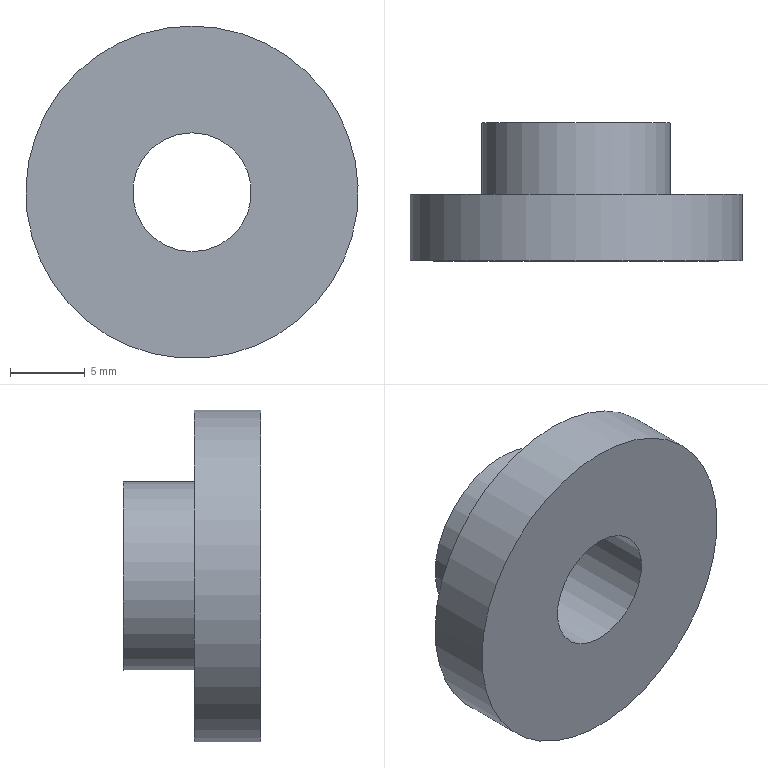Part | NX | features piston hat 2 | 1 solid | 8 faces | box 22.225 x 9.22 x 22.225 mm | volume 1664 mm3 | plane 4 | cylinder 4 | commonest cylinder face diameters 7.95 x1 12.649 x1 19.05 x1 22.225 x1
STEP:
#1=CARTESIAN_POINT('',(0.,-31.073,3.975));
#2=VERTEX_POINT('',#1);
#3=CARTESIAN_POINT('',(0.,-31.073,0.));
#4=DIRECTION('',(0.,1.,0.));
#5=DIRECTION('',(0.,0.,1.));
#6=AXIS2_PLACEMENT_3D('',#3,#4,#5);
#7=CIRCLE('',#6,3.975);
#8=EDGE_CURVE('',#2,#2,#7,.T.);
#9=ORIENTED_EDGE('',*,*,#8,.F.);
#10=EDGE_LOOP('',(#9));
#11=FACE_BOUND('',#10,.T.);
#12=CARTESIAN_POINT('',(0.,-31.073,6.325));
#13=VERTEX_POINT('',#12);
#14=CARTESIAN_POINT('',(0.,-31.073,0.));
#15=DIRECTION('',(0.,1.,0.));
#16=DIRECTION('',(0.,0.,1.));
#17=AXIS2_PLACEMENT_3D('',#14,#15,#16);
#18=CIRCLE('',#17,6.325);
#19=EDGE_CURVE('',#13,#13,#18,.T.);
#20=ORIENTED_EDGE('',*,*,#19,.T.);
#21=EDGE_LOOP('',(#20));
#22=FACE_BOUND('',#21,.T.);
#23=CARTESIAN_POINT('',(3.975,-31.073,0.));
#24=DIRECTION('',(0.,-1.,0.));
#25=DIRECTION('',(0.,0.,-1.));
#26=AXIS2_PLACEMENT_3D('',#23,#24,#25);
#27=PLANE('',#26);
#28=ADVANCED_FACE('',(#11,#22),#27,.F.);
#29=CARTESIAN_POINT('',(0.,-40.293,3.975));
#30=VERTEX_POINT('',#29);
#31=CARTESIAN_POINT('',(0.,-40.293,0.));
#32=DIRECTION('',(0.,1.,0.));
#33=DIRECTION('',(0.,0.,1.));
#34=AXIS2_PLACEMENT_3D('',#31,#32,#33);
#35=CIRCLE('',#34,3.975);
#36=EDGE_CURVE('',#30,#30,#35,.T.);
#37=ORIENTED_EDGE('',*,*,#36,.F.);
#38=EDGE_LOOP('',(#37));
#39=FACE_BOUND('',#38,.T.);
#40=ORIENTED_EDGE('',*,*,#8,.T.);
#41=EDGE_LOOP('',(#40));
#42=FACE_BOUND('',#41,.T.);
#43=CARTESIAN_POINT('',(0.,42.699,0.));
#44=DIRECTION('',(0.,1.,0.));
#45=DIRECTION('',(0.,0.,1.));
#46=AXIS2_PLACEMENT_3D('',#43,#44,#45);
#47=CYLINDRICAL_SURFACE('',#46,3.975);
#48=ADVANCED_FACE('',(#39,#42),#47,.F.);
#49=CARTESIAN_POINT('',(0.,-40.293,11.113));
#50=VERTEX_POINT('',#49);
#51=CARTESIAN_POINT('',(0.,-40.293,0.));
#52=DIRECTION('',(0.,1.,0.));
#53=DIRECTION('',(0.,0.,1.));
#54=AXIS2_PLACEMENT_3D('',#51,#52,#53);
#55=CIRCLE('',#54,11.113);
#56=EDGE_CURVE('',#50,#50,#55,.T.);
#57=ORIENTED_EDGE('',*,*,#56,.F.);
#58=EDGE_LOOP('',(#57));
#59=FACE_BOUND('',#58,.T.);
#60=ORIENTED_EDGE('',*,*,#36,.T.);
#61=EDGE_LOOP('',(#60));
#62=FACE_BOUND('',#61,.T.);
#63=CARTESIAN_POINT('',(11.113,-40.293,0.));
#64=DIRECTION('',(0.,1.,0.));
#65=DIRECTION('',(0.,0.,1.));
#66=AXIS2_PLACEMENT_3D('',#63,#64,#65);
#67=PLANE('',#66);
#68=ADVANCED_FACE('',(#59,#62),#67,.F.);
#69=CARTESIAN_POINT('',(0.,-35.848,11.113));
#70=VERTEX_POINT('',#69);
#71=CARTESIAN_POINT('',(0.,-35.848,0.));
#72=DIRECTION('',(0.,1.,0.));
#73=DIRECTION('',(0.,0.,1.));
#74=AXIS2_PLACEMENT_3D('',#71,#72,#73);
#75=CIRCLE('',#74,11.113);
#76=EDGE_CURVE('',#70,#70,#75,.T.);
#77=ORIENTED_EDGE('',*,*,#76,.F.);
#78=EDGE_LOOP('',(#77));
#79=FACE_BOUND('',#78,.T.);
#80=ORIENTED_EDGE('',*,*,#56,.T.);
#81=EDGE_LOOP('',(#80));
#82=FACE_BOUND('',#81,.T.);
#83=CARTESIAN_POINT('',(0.,42.699,0.));
#84=DIRECTION('',(0.,1.,0.));
#85=DIRECTION('',(0.,0.,1.));
#86=AXIS2_PLACEMENT_3D('',#83,#84,#85);
#87=CYLINDRICAL_SURFACE('',#86,11.113);
#88=ADVANCED_FACE('',(#79,#82),#87,.T.);
#89=CARTESIAN_POINT('',(0.,-35.848,9.525));
#90=VERTEX_POINT('',#89);
#91=CARTESIAN_POINT('',(0.,-35.848,0.));
#92=DIRECTION('',(0.,1.,0.));
#93=DIRECTION('',(0.,0.,1.));
#94=AXIS2_PLACEMENT_3D('',#91,#92,#93);
#95=CIRCLE('',#94,9.525);
#96=EDGE_CURVE('',#90,#90,#95,.T.);
#97=ORIENTED_EDGE('',*,*,#96,.F.);
#98=EDGE_LOOP('',(#97));
#99=FACE_BOUND('',#98,.T.);
#100=ORIENTED_EDGE('',*,*,#76,.T.);
#101=EDGE_LOOP('',(#100));
#102=FACE_BOUND('',#101,.T.);
#103=CARTESIAN_POINT('',(9.525,-35.848,0.));
#104=DIRECTION('',(0.,-1.,0.));
#105=DIRECTION('',(0.,0.,-1.));
#106=AXIS2_PLACEMENT_3D('',#103,#104,#105);
#107=PLANE('',#106);
#108=ADVANCED_FACE('',(#99,#102),#107,.F.);
#109=CARTESIAN_POINT('',(0.,-37.118,9.525));
#110=VERTEX_POINT('',#109);
#111=CARTESIAN_POINT('',(0.,-37.118,0.));
#112=DIRECTION('',(0.,1.,0.));
#113=DIRECTION('',(0.,0.,1.));
#114=AXIS2_PLACEMENT_3D('',#111,#112,#113);
#115=CIRCLE('',#114,9.525);
#116=EDGE_CURVE('',#110,#110,#115,.T.);
#117=ORIENTED_EDGE('',*,*,#116,.F.);
#118=EDGE_LOOP('',(#117));
#119=FACE_BOUND('',#118,.T.);
#120=ORIENTED_EDGE('',*,*,#96,.T.);
#121=EDGE_LOOP('',(#120));
#122=FACE_BOUND('',#121,.T.);
#123=CARTESIAN_POINT('',(0.,42.699,0.));
#124=DIRECTION('',(0.,1.,0.));
#125=DIRECTION('',(0.,0.,1.));
#126=AXIS2_PLACEMENT_3D('',#123,#124,#125);
#127=CYLINDRICAL_SURFACE('',#126,9.525);
#128=ADVANCED_FACE('',(#119,#122),#127,.F.);
#129=CARTESIAN_POINT('',(0.,-37.118,6.325));
#130=VERTEX_POINT('',#129);
#131=CARTESIAN_POINT('',(0.,-37.118,0.));
#132=DIRECTION('',(0.,1.,0.));
#133=DIRECTION('',(0.,0.,1.));
#134=AXIS2_PLACEMENT_3D('',#131,#132,#133);
#135=CIRCLE('',#134,6.325);
#136=EDGE_CURVE('',#130,#130,#135,.T.);
#137=ORIENTED_EDGE('',*,*,#136,.F.);
#138=EDGE_LOOP('',(#137));
#139=FACE_BOUND('',#138,.T.);
#140=ORIENTED_EDGE('',*,*,#116,.T.);
#141=EDGE_LOOP('',(#140));
#142=FACE_BOUND('',#141,.T.);
#143=CARTESIAN_POINT('',(6.325,-37.118,0.));
#144=DIRECTION('',(0.,-1.,0.));
#145=DIRECTION('',(0.,0.,-1.));
#146=AXIS2_PLACEMENT_3D('',#143,#144,#145);
#147=PLANE('',#146);
#148=ADVANCED_FACE('',(#139,#142),#147,.F.);
#149=ORIENTED_EDGE('',*,*,#19,.F.);
#150=EDGE_LOOP('',(#149));
#151=FACE_BOUND('',#150,.T.);
#152=ORIENTED_EDGE('',*,*,#136,.T.);
#153=EDGE_LOOP('',(#152));
#154=FACE_BOUND('',#153,.T.);
#155=CARTESIAN_POINT('',(0.,42.699,0.));
#156=DIRECTION('',(0.,1.,0.));
#157=DIRECTION('',(0.,0.,1.));
#158=AXIS2_PLACEMENT_3D('',#155,#156,#157);
#159=CYLINDRICAL_SURFACE('',#158,6.325);
#160=ADVANCED_FACE('',(#151,#154),#159,.T.);
#161=CLOSED_SHELL('',(#28,#48,#68,#88,#108,#128,#148,#160));
#162=MANIFOLD_SOLID_BREP('',#161);
#163=(LENGTH_UNIT()NAMED_UNIT(*)SI_UNIT(.MILLI.,.METRE.));
#164=UNCERTAINTY_MEASURE_WITH_UNIT(LENGTH_MEASURE(0.00001),#163,'','');
#165=(NAMED_UNIT(*)PLANE_ANGLE_UNIT()SI_UNIT($,.RADIAN.));
#166=(NAMED_UNIT(*)SI_UNIT($,.STERADIAN.)SOLID_ANGLE_UNIT());
#167=(GEOMETRIC_REPRESENTATION_CONTEXT(3)GLOBAL_UNCERTAINTY_ASSIGNED_CONTEXT((#164))GLOBAL_UNIT_ASSIGNED_CONTEXT((#163,#165,#166))REPRESENTATION_CONTEXT('',''));
#168=ADVANCED_BREP_SHAPE_REPRESENTATION('',(#162),#167);